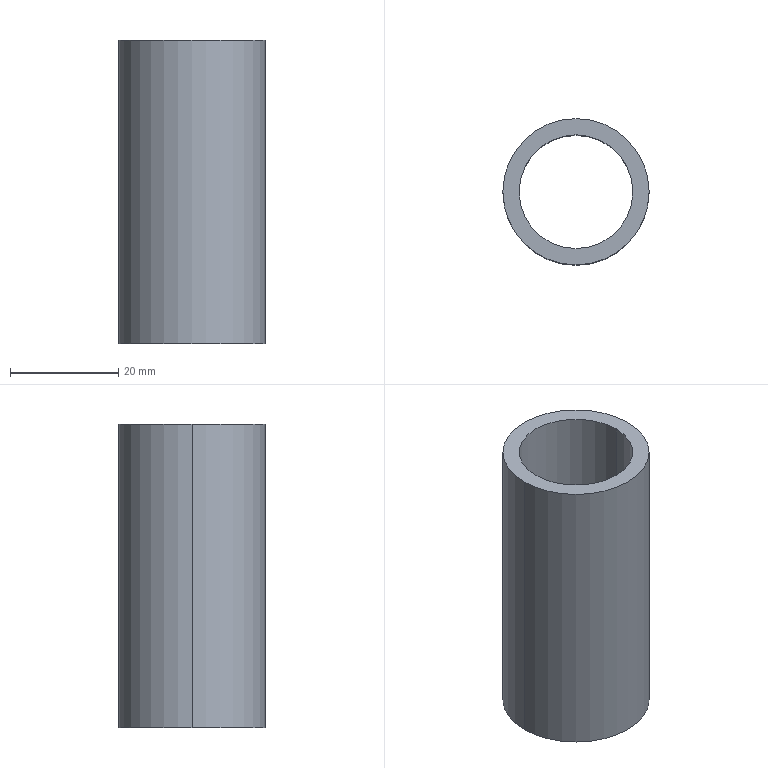Part | SolidWorks | features Extrusion 1 | 1 solid | 6 faces | box 27 x 27 x 56 mm | volume 12667 mm3 | cylinder 4 | plane 2 | commonest cylinder face diameters 21 x2 27 x2
STEP:
#1=CARTESIAN_POINT('',(-10.5,0.,28.));
#2=VERTEX_POINT('',#1);
#3=CARTESIAN_POINT('',(10.5,0.,28.));
#4=VERTEX_POINT('',#3);
#5=CARTESIAN_POINT('',(0.,0.,28.));
#6=DIRECTION('',(0.,0.,1.));
#7=DIRECTION('',(1.,0.,0.));
#8=AXIS2_PLACEMENT_3D('',#5,#6,#7);
#9=CIRCLE('',#8,10.5);
#10=EDGE_CURVE('',#2,#4,#9,.T.);
#11=ORIENTED_EDGE('',*,*,#10,.T.);
#12=CARTESIAN_POINT('',(10.5,0.,-28.));
#13=VERTEX_POINT('',#12);
#14=CARTESIAN_POINT('',(10.5,0.,28.));
#15=DIRECTION('',(0.,0.,-1.));
#16=VECTOR('',#15,1000.);
#17=LINE('',#14,#16);
#18=EDGE_CURVE('',#4,#13,#17,.T.);
#19=ORIENTED_EDGE('',*,*,#18,.T.);
#20=CARTESIAN_POINT('',(-10.5,0.,-28.));
#21=VERTEX_POINT('',#20);
#22=CARTESIAN_POINT('',(0.,0.,-28.));
#23=DIRECTION('',(0.,0.,1.));
#24=DIRECTION('',(1.,0.,0.));
#25=AXIS2_PLACEMENT_3D('',#22,#23,#24);
#26=CIRCLE('',#25,10.5);
#27=EDGE_CURVE('',#21,#13,#26,.T.);
#28=ORIENTED_EDGE('',*,*,#27,.F.);
#29=CARTESIAN_POINT('',(-10.5,0.,28.));
#30=DIRECTION('',(0.,0.,-1.));
#31=VECTOR('',#30,1000.);
#32=LINE('',#29,#31);
#33=EDGE_CURVE('',#2,#21,#32,.T.);
#34=ORIENTED_EDGE('',*,*,#33,.F.);
#35=EDGE_LOOP('',(#11,#19,#28,#34));
#36=FACE_OUTER_BOUND('',#35,.T.);
#37=CARTESIAN_POINT('',(0.,0.,28.));
#38=DIRECTION('',(0.,0.,-1.));
#39=DIRECTION('',(-1.,0.,0.));
#40=AXIS2_PLACEMENT_3D('',#37,#38,#39);
#41=CYLINDRICAL_SURFACE('',#40,10.5);
#42=ADVANCED_FACE('',(#36),#41,.F.);
#43=CARTESIAN_POINT('',(13.5,0.,28.));
#44=VERTEX_POINT('',#43);
#45=CARTESIAN_POINT('',(-13.5,0.,28.));
#46=VERTEX_POINT('',#45);
#47=CARTESIAN_POINT('',(0.,0.,28.));
#48=DIRECTION('',(0.,0.,1.));
#49=DIRECTION('',(1.,0.,0.));
#50=AXIS2_PLACEMENT_3D('',#47,#48,#49);
#51=CIRCLE('',#50,13.5);
#52=EDGE_CURVE('',#44,#46,#51,.T.);
#53=ORIENTED_EDGE('',*,*,#52,.F.);
#54=CARTESIAN_POINT('',(13.5,0.,-28.));
#55=VERTEX_POINT('',#54);
#56=CARTESIAN_POINT('',(13.5,0.,28.));
#57=DIRECTION('',(0.,0.,-1.));
#58=VECTOR('',#57,1000.);
#59=LINE('',#56,#58);
#60=EDGE_CURVE('',#44,#55,#59,.T.);
#61=ORIENTED_EDGE('',*,*,#60,.T.);
#62=CARTESIAN_POINT('',(-13.5,0.,-28.));
#63=VERTEX_POINT('',#62);
#64=CARTESIAN_POINT('',(0.,0.,-28.));
#65=DIRECTION('',(0.,0.,1.));
#66=DIRECTION('',(1.,0.,0.));
#67=AXIS2_PLACEMENT_3D('',#64,#65,#66);
#68=CIRCLE('',#67,13.5);
#69=EDGE_CURVE('',#55,#63,#68,.T.);
#70=ORIENTED_EDGE('',*,*,#69,.T.);
#71=CARTESIAN_POINT('',(-13.5,0.,28.));
#72=DIRECTION('',(0.,0.,-1.));
#73=VECTOR('',#72,1000.);
#74=LINE('',#71,#73);
#75=EDGE_CURVE('',#46,#63,#74,.T.);
#76=ORIENTED_EDGE('',*,*,#75,.F.);
#77=EDGE_LOOP('',(#53,#61,#70,#76));
#78=FACE_OUTER_BOUND('',#77,.T.);
#79=CARTESIAN_POINT('',(0.,0.,28.));
#80=DIRECTION('',(0.,0.,-1.));
#81=DIRECTION('',(-1.,0.,0.));
#82=AXIS2_PLACEMENT_3D('',#79,#80,#81);
#83=CYLINDRICAL_SURFACE('',#82,13.5);
#84=ADVANCED_FACE('',(#78),#83,.T.);
#85=CARTESIAN_POINT('',(0.,0.,28.));
#86=DIRECTION('',(0.,0.,1.));
#87=DIRECTION('',(1.,0.,0.));
#88=AXIS2_PLACEMENT_3D('',#85,#86,#87);
#89=CIRCLE('',#88,13.5);
#90=EDGE_CURVE('',#46,#44,#89,.T.);
#91=ORIENTED_EDGE('',*,*,#90,.T.);
#92=ORIENTED_EDGE('',*,*,#52,.T.);
#93=EDGE_LOOP('',(#91,#92));
#94=FACE_OUTER_BOUND('',#93,.T.);
#95=ORIENTED_EDGE('',*,*,#10,.F.);
#96=CARTESIAN_POINT('',(0.,0.,28.));
#97=DIRECTION('',(0.,0.,1.));
#98=DIRECTION('',(1.,0.,0.));
#99=AXIS2_PLACEMENT_3D('',#96,#97,#98);
#100=CIRCLE('',#99,10.5);
#101=EDGE_CURVE('',#4,#2,#100,.T.);
#102=ORIENTED_EDGE('',*,*,#101,.F.);
#103=EDGE_LOOP('',(#95,#102));
#104=FACE_BOUND('',#103,.T.);
#105=CARTESIAN_POINT('',(0.,0.,28.));
#106=DIRECTION('',(0.,0.,1.));
#107=DIRECTION('',(1.,0.,0.));
#108=AXIS2_PLACEMENT_3D('',#105,#106,#107);
#109=PLANE('',#108);
#110=ADVANCED_FACE('',(#94,#104),#109,.T.);
#111=CARTESIAN_POINT('',(0.,0.,-28.));
#112=DIRECTION('',(0.,0.,1.));
#113=DIRECTION('',(1.,0.,0.));
#114=AXIS2_PLACEMENT_3D('',#111,#112,#113);
#115=CIRCLE('',#114,13.5);
#116=EDGE_CURVE('',#63,#55,#115,.T.);
#117=ORIENTED_EDGE('',*,*,#116,.F.);
#118=ORIENTED_EDGE('',*,*,#69,.F.);
#119=EDGE_LOOP('',(#117,#118));
#120=FACE_OUTER_BOUND('',#119,.T.);
#121=ORIENTED_EDGE('',*,*,#27,.T.);
#122=CARTESIAN_POINT('',(0.,0.,-28.));
#123=DIRECTION('',(0.,0.,1.));
#124=DIRECTION('',(1.,0.,0.));
#125=AXIS2_PLACEMENT_3D('',#122,#123,#124);
#126=CIRCLE('',#125,10.5);
#127=EDGE_CURVE('',#13,#21,#126,.T.);
#128=ORIENTED_EDGE('',*,*,#127,.T.);
#129=EDGE_LOOP('',(#121,#128));
#130=FACE_BOUND('',#129,.T.);
#131=CARTESIAN_POINT('',(0.,0.,-28.));
#132=DIRECTION('',(0.,0.,1.));
#133=DIRECTION('',(1.,0.,0.));
#134=AXIS2_PLACEMENT_3D('',#131,#132,#133);
#135=PLANE('',#134);
#136=ADVANCED_FACE('',(#120,#130),#135,.F.);
#137=ORIENTED_EDGE('',*,*,#60,.F.);
#138=ORIENTED_EDGE('',*,*,#90,.F.);
#139=ORIENTED_EDGE('',*,*,#75,.T.);
#140=ORIENTED_EDGE('',*,*,#116,.T.);
#141=EDGE_LOOP('',(#137,#138,#139,#140));
#142=FACE_OUTER_BOUND('',#141,.T.);
#143=CARTESIAN_POINT('',(0.,0.,28.));
#144=DIRECTION('',(0.,0.,-1.));
#145=DIRECTION('',(-1.,0.,0.));
#146=AXIS2_PLACEMENT_3D('',#143,#144,#145);
#147=CYLINDRICAL_SURFACE('',#146,13.5);
#148=ADVANCED_FACE('',(#142),#147,.T.);
#149=ORIENTED_EDGE('',*,*,#18,.F.);
#150=ORIENTED_EDGE('',*,*,#101,.T.);
#151=ORIENTED_EDGE('',*,*,#33,.T.);
#152=ORIENTED_EDGE('',*,*,#127,.F.);
#153=EDGE_LOOP('',(#149,#150,#151,#152));
#154=FACE_OUTER_BOUND('',#153,.T.);
#155=CARTESIAN_POINT('',(0.,0.,28.));
#156=DIRECTION('',(0.,0.,-1.));
#157=DIRECTION('',(-1.,0.,0.));
#158=AXIS2_PLACEMENT_3D('',#155,#156,#157);
#159=CYLINDRICAL_SURFACE('',#158,10.5);
#160=ADVANCED_FACE('',(#154),#159,.F.);
#161=CLOSED_SHELL('',(#42,#84,#110,#136,#148,#160));
#162=MANIFOLD_SOLID_BREP('',#161);
#163=CARTESIAN_POINT('',(0.,0.,0.));
#164=DIRECTION('',(0.,0.,1.));
#165=DIRECTION('',(1.,0.,0.));
#166=AXIS2_PLACEMENT_3D('',#163,#164,#165);
#167=(LENGTH_UNIT()NAMED_UNIT(*)SI_UNIT(.MILLI.,.METRE.));
#168=UNCERTAINTY_MEASURE_WITH_UNIT(LENGTH_MEASURE(0.00001),#167,'','');
#169=(NAMED_UNIT(*)PLANE_ANGLE_UNIT()SI_UNIT($,.RADIAN.));
#170=(NAMED_UNIT(*)SI_UNIT($,.STERADIAN.)SOLID_ANGLE_UNIT());
#171=(GEOMETRIC_REPRESENTATION_CONTEXT(3)GLOBAL_UNCERTAINTY_ASSIGNED_CONTEXT((#168))GLOBAL_UNIT_ASSIGNED_CONTEXT((#167,#169,#170))REPRESENTATION_CONTEXT('',''));
#172=ADVANCED_BREP_SHAPE_REPRESENTATION('',(#162,#166),#171);